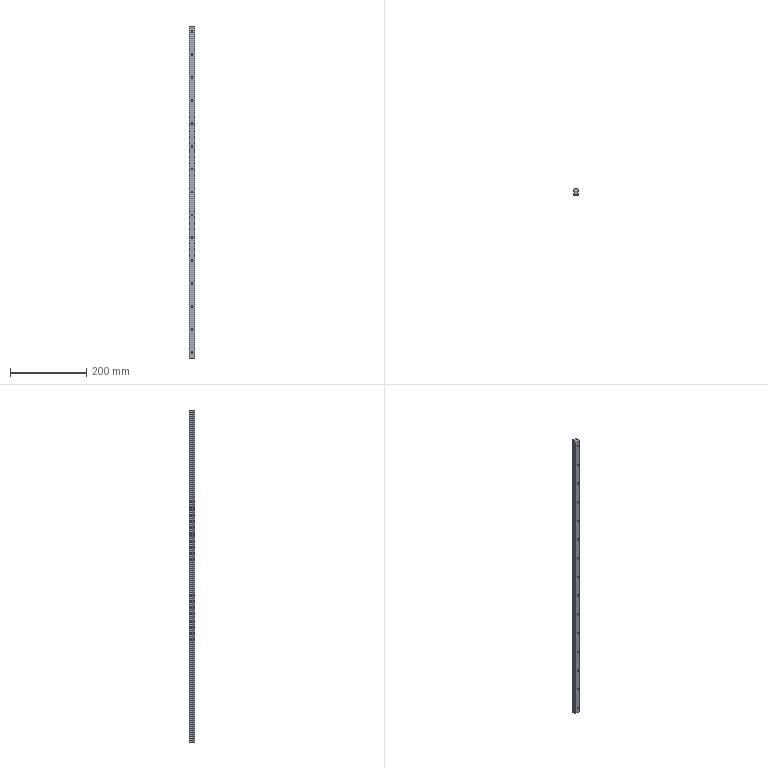Part | STEP file | HGR15-rail L870 | 1 solid | 111 faces | box 15 x 15 x 870 mm | volume 160134 mm3 | cylinder 74 | plane 37 | commonest cylinder face diameters 4.5 x30 7.5 x30 0.8 x8 3.24 x4 2 x2